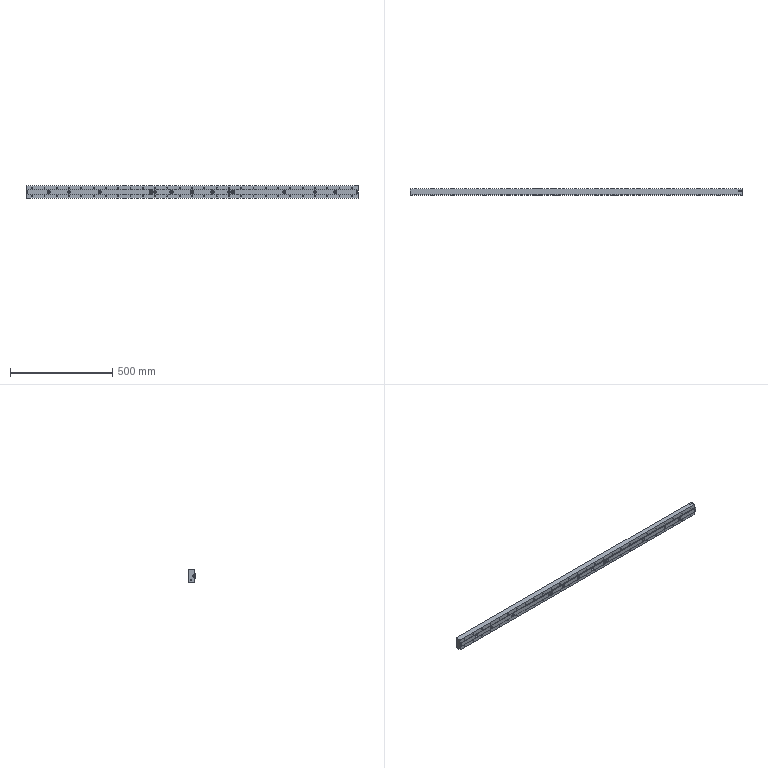Part | STEP file | rail fixing plate | 1 solid | 203 faces | box 1620 x 30 x 60 mm | volume 2595354 mm3 | cylinder 168 | plane 19 | cone 16 | commonest cylinder face diameters 4.2 x116 9 x18 15 x18 3.3 x8 12 x8